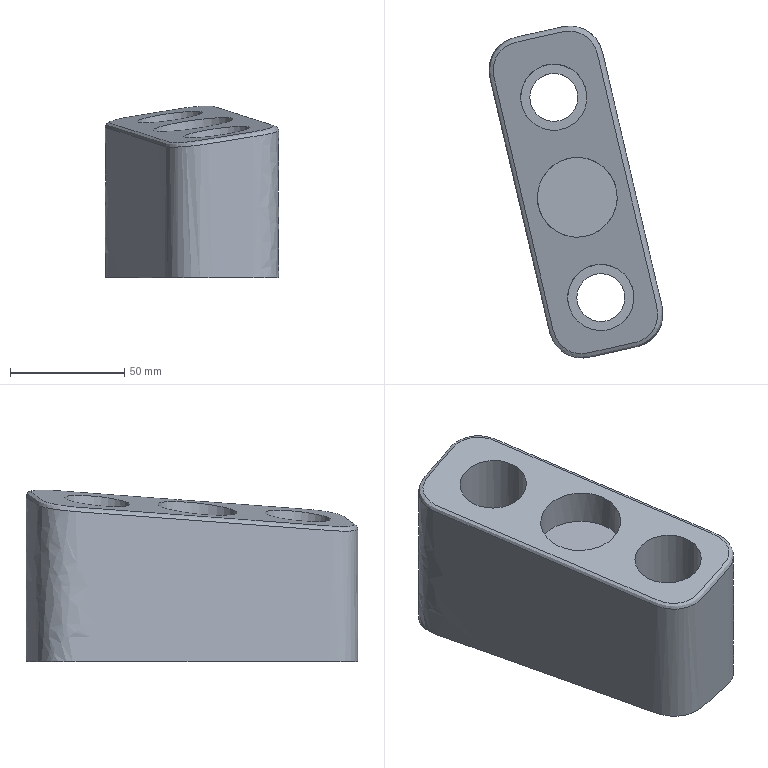Part | NX | features solid 2 | 1 solid | 12 faces | box 75.921 x 145.178 x 75.298 mm | volume 388024 mm3 | cylinder 5 | plane 4 | spline 3 | commonest cylinder face diameters 21 x2 29 x2 35 x1